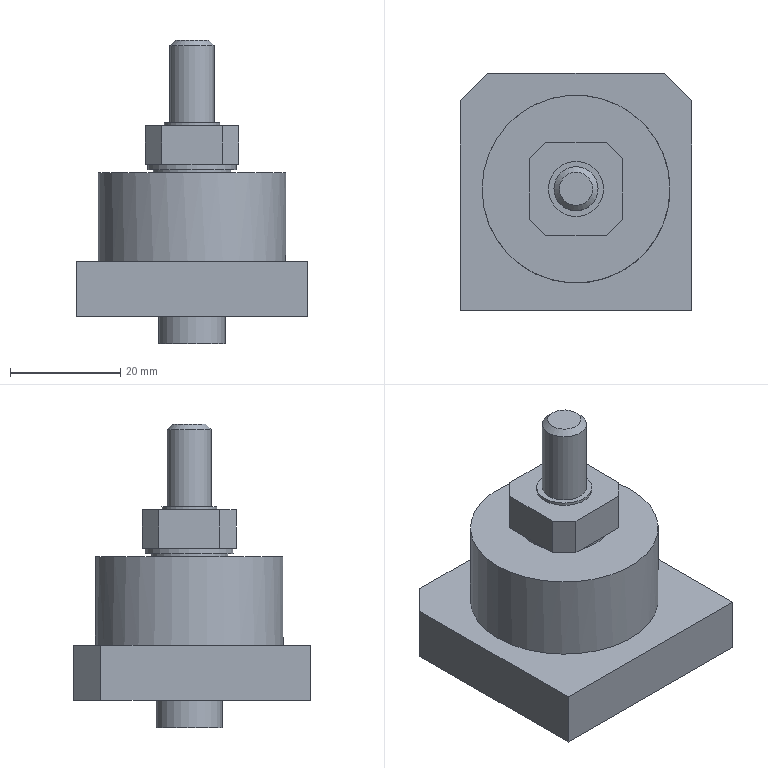Part | NX | features EXTRUDE 8, DATUM_CSYS 7, SKETCH 6, CHAMFER 3, OFFSET 1 | 1 solid | 30 faces | box 42 x 43 x 55 mm | volume 35859 mm3 | plane 23 | cylinder 6 | cone 1 | commonest cylinder face diameters 8 x1 10 x1 12 x1 14 x1 16 x1 34 x1
STEP:
#1=CARTESIAN_POINT('',(0.,16.,0.));
#2=VERTEX_POINT('',#1);
#3=CARTESIAN_POINT('',(0.,-22.,0.));
#4=VERTEX_POINT('',#3);
#5=CARTESIAN_POINT('',(0.,21.,0.));
#6=DIRECTION('',(0.,-1.,0.));
#7=VECTOR('',#6,1000.);
#8=LINE('',#5,#7);
#9=EDGE_CURVE('',#2,#4,#8,.T.);
#10=ORIENTED_EDGE('',*,*,#9,.F.);
#11=CARTESIAN_POINT('',(0.,16.,10.));
#12=VERTEX_POINT('',#11);
#13=CARTESIAN_POINT('',(0.,16.,10.));
#14=DIRECTION('',(0.,0.,1.));
#15=VECTOR('',#14,1000.);
#16=LINE('',#13,#15);
#17=EDGE_CURVE('',#2,#12,#16,.T.);
#18=ORIENTED_EDGE('',*,*,#17,.T.);
#19=CARTESIAN_POINT('',(0.,-22.,10.));
#20=VERTEX_POINT('',#19);
#21=CARTESIAN_POINT('',(0.,21.,10.));
#22=DIRECTION('',(0.,-1.,0.));
#23=VECTOR('',#22,1000.);
#24=LINE('',#21,#23);
#25=EDGE_CURVE('',#12,#20,#24,.T.);
#26=ORIENTED_EDGE('',*,*,#25,.T.);
#27=CARTESIAN_POINT('',(0.,-22.,10.));
#28=DIRECTION('',(0.,0.,-1.));
#29=VECTOR('',#28,1000.);
#30=LINE('',#27,#29);
#31=EDGE_CURVE('',#20,#4,#30,.T.);
#32=ORIENTED_EDGE('',*,*,#31,.T.);
#33=EDGE_LOOP('',(#10,#18,#26,#32));
#34=FACE_BOUND('',#33,.T.);
#35=CARTESIAN_POINT('',(0.,21.,10.));
#36=DIRECTION('',(1.,0.,0.));
#37=DIRECTION('',(0.,1.,0.));
#38=AXIS2_PLACEMENT_3D('',#35,#36,#37);
#39=PLANE('',#38);
#40=ADVANCED_FACE('',(#34),#39,.T.);
#41=CARTESIAN_POINT('',(-42.,-22.,0.));
#42=VERTEX_POINT('',#41);
#43=CARTESIAN_POINT('',(0.,-22.,0.));
#44=DIRECTION('',(-1.,0.,0.));
#45=VECTOR('',#44,1000.);
#46=LINE('',#43,#45);
#47=EDGE_CURVE('',#4,#42,#46,.T.);
#48=ORIENTED_EDGE('',*,*,#47,.F.);
#49=ORIENTED_EDGE('',*,*,#31,.F.);
#50=CARTESIAN_POINT('',(-42.,-22.,10.));
#51=VERTEX_POINT('',#50);
#52=CARTESIAN_POINT('',(0.,-22.,10.));
#53=DIRECTION('',(-1.,0.,0.));
#54=VECTOR('',#53,1000.);
#55=LINE('',#52,#54);
#56=EDGE_CURVE('',#20,#51,#55,.T.);
#57=ORIENTED_EDGE('',*,*,#56,.T.);
#58=CARTESIAN_POINT('',(-42.,-22.,10.));
#59=DIRECTION('',(0.,0.,-1.));
#60=VECTOR('',#59,1000.);
#61=LINE('',#58,#60);
#62=EDGE_CURVE('',#51,#42,#61,.T.);
#63=ORIENTED_EDGE('',*,*,#62,.T.);
#64=EDGE_LOOP('',(#48,#49,#57,#63));
#65=FACE_BOUND('',#64,.T.);
#66=CARTESIAN_POINT('',(0.,-22.,10.));
#67=DIRECTION('',(0.,-1.,0.));
#68=DIRECTION('',(1.,0.,0.));
#69=AXIS2_PLACEMENT_3D('',#66,#67,#68);
#70=PLANE('',#69);
#71=ADVANCED_FACE('',(#65),#70,.T.);
#72=CARTESIAN_POINT('',(-42.,16.,10.));
#73=VERTEX_POINT('',#72);
#74=CARTESIAN_POINT('',(-42.,-21.,10.));
#75=DIRECTION('',(0.,1.,0.));
#76=VECTOR('',#75,1000.);
#77=LINE('',#74,#76);
#78=EDGE_CURVE('',#51,#73,#77,.T.);
#79=ORIENTED_EDGE('',*,*,#78,.T.);
#80=CARTESIAN_POINT('',(-42.,16.,0.));
#81=VERTEX_POINT('',#80);
#82=CARTESIAN_POINT('',(-42.,16.,10.));
#83=DIRECTION('',(0.,0.,-1.));
#84=VECTOR('',#83,1000.);
#85=LINE('',#82,#84);
#86=EDGE_CURVE('',#73,#81,#85,.T.);
#87=ORIENTED_EDGE('',*,*,#86,.T.);
#88=CARTESIAN_POINT('',(-42.,-21.,0.));
#89=DIRECTION('',(0.,1.,0.));
#90=VECTOR('',#89,1000.);
#91=LINE('',#88,#90);
#92=EDGE_CURVE('',#42,#81,#91,.T.);
#93=ORIENTED_EDGE('',*,*,#92,.F.);
#94=ORIENTED_EDGE('',*,*,#62,.F.);
#95=EDGE_LOOP('',(#79,#87,#93,#94));
#96=FACE_BOUND('',#95,.T.);
#97=CARTESIAN_POINT('',(-42.,-21.,10.));
#98=DIRECTION('',(-1.,0.,0.));
#99=DIRECTION('',(0.,0.,1.));
#100=AXIS2_PLACEMENT_3D('',#97,#98,#99);
#101=PLANE('',#100);
#102=ADVANCED_FACE('',(#96),#101,.T.);
#103=CARTESIAN_POINT('',(-37.,21.,10.));
#104=VERTEX_POINT('',#103);
#105=CARTESIAN_POINT('',(-5.,21.,10.));
#106=VERTEX_POINT('',#105);
#107=CARTESIAN_POINT('',(-42.,21.,10.));
#108=DIRECTION('',(1.,0.,0.));
#109=VECTOR('',#108,1000.);
#110=LINE('',#107,#109);
#111=EDGE_CURVE('',#104,#106,#110,.T.);
#112=ORIENTED_EDGE('',*,*,#111,.T.);
#113=CARTESIAN_POINT('',(-5.,21.,0.));
#114=VERTEX_POINT('',#113);
#115=CARTESIAN_POINT('',(-5.,21.,10.));
#116=DIRECTION('',(0.,0.,-1.));
#117=VECTOR('',#116,1000.);
#118=LINE('',#115,#117);
#119=EDGE_CURVE('',#106,#114,#118,.T.);
#120=ORIENTED_EDGE('',*,*,#119,.T.);
#121=CARTESIAN_POINT('',(-37.,21.,0.));
#122=VERTEX_POINT('',#121);
#123=CARTESIAN_POINT('',(-42.,21.,0.));
#124=DIRECTION('',(1.,0.,0.));
#125=VECTOR('',#124,1000.);
#126=LINE('',#123,#125);
#127=EDGE_CURVE('',#122,#114,#126,.T.);
#128=ORIENTED_EDGE('',*,*,#127,.F.);
#129=CARTESIAN_POINT('',(-37.,21.,10.));
#130=DIRECTION('',(0.,0.,1.));
#131=VECTOR('',#130,1000.);
#132=LINE('',#129,#131);
#133=EDGE_CURVE('',#122,#104,#132,.T.);
#134=ORIENTED_EDGE('',*,*,#133,.T.);
#135=EDGE_LOOP('',(#112,#120,#128,#134));
#136=FACE_BOUND('',#135,.T.);
#137=CARTESIAN_POINT('',(-42.,21.,10.));
#138=DIRECTION('',(0.,1.,0.));
#139=DIRECTION('',(0.,0.,1.));
#140=AXIS2_PLACEMENT_3D('',#137,#138,#139);
#141=PLANE('',#140);
#142=ADVANCED_FACE('',(#136),#141,.T.);
#143=CARTESIAN_POINT('',(-38.,0.,10.));
#144=VERTEX_POINT('',#143);
#145=CARTESIAN_POINT('',(-21.,0.,10.));
#146=DIRECTION('',(0.,0.,-1.));
#147=DIRECTION('',(-1.,0.,0.));
#148=AXIS2_PLACEMENT_3D('',#145,#146,#147);
#149=CIRCLE('',#148,17.);
#150=EDGE_CURVE('',#144,#144,#149,.T.);
#151=ORIENTED_EDGE('',*,*,#150,.T.);
#152=EDGE_LOOP('',(#151));
#153=FACE_BOUND('',#152,.T.);
#154=ORIENTED_EDGE('',*,*,#25,.F.);
#155=CARTESIAN_POINT('',(-5.,21.,10.));
#156=DIRECTION('',(0.7071,-0.7071,0.));
#157=VECTOR('',#156,1000.);
#158=LINE('',#155,#157);
#159=EDGE_CURVE('',#12,#106,#158,.F.);
#160=ORIENTED_EDGE('',*,*,#159,.T.);
#161=ORIENTED_EDGE('',*,*,#111,.F.);
#162=CARTESIAN_POINT('',(-42.,16.,10.));
#163=DIRECTION('',(0.7071,0.7071,0.));
#164=VECTOR('',#163,1000.);
#165=LINE('',#162,#164);
#166=EDGE_CURVE('',#104,#73,#165,.F.);
#167=ORIENTED_EDGE('',*,*,#166,.T.);
#168=ORIENTED_EDGE('',*,*,#78,.F.);
#169=ORIENTED_EDGE('',*,*,#56,.F.);
#170=EDGE_LOOP('',(#154,#160,#161,#167,#168,#169));
#171=FACE_BOUND('',#170,.T.);
#172=CARTESIAN_POINT('',(0.,0.,10.));
#173=DIRECTION('',(0.,0.,-1.));
#174=DIRECTION('',(-1.,0.,0.));
#175=AXIS2_PLACEMENT_3D('',#172,#173,#174);
#176=PLANE('',#175);
#177=ADVANCED_FACE('',(#153,#171),#176,.F.);
#178=CARTESIAN_POINT('',(-27.,0.,0.));
#179=VERTEX_POINT('',#178);
#180=CARTESIAN_POINT('',(-21.,0.,0.));
#181=DIRECTION('',(0.,0.,-1.));
#182=DIRECTION('',(-1.,0.,0.));
#183=AXIS2_PLACEMENT_3D('',#180,#181,#182);
#184=CIRCLE('',#183,6.);
#185=EDGE_CURVE('',#179,#179,#184,.F.);
#186=ORIENTED_EDGE('',*,*,#185,.T.);
#187=EDGE_LOOP('',(#186));
#188=FACE_BOUND('',#187,.T.);
#189=ORIENTED_EDGE('',*,*,#127,.T.);
#190=CARTESIAN_POINT('',(8.,8.,0.));
#191=DIRECTION('',(-0.7071,0.7071,0.));
#192=VECTOR('',#191,1000.);
#193=LINE('',#190,#192);
#194=EDGE_CURVE('',#114,#2,#193,.F.);
#195=ORIENTED_EDGE('',*,*,#194,.T.);
#196=ORIENTED_EDGE('',*,*,#9,.T.);
#197=ORIENTED_EDGE('',*,*,#47,.T.);
#198=ORIENTED_EDGE('',*,*,#92,.T.);
#199=CARTESIAN_POINT('',(-29.,29.,0.));
#200=DIRECTION('',(-0.7071,-0.7071,0.));
#201=VECTOR('',#200,1000.);
#202=LINE('',#199,#201);
#203=EDGE_CURVE('',#81,#122,#202,.F.);
#204=ORIENTED_EDGE('',*,*,#203,.T.);
#205=EDGE_LOOP('',(#189,#195,#196,#197,#198,#204));
#206=FACE_BOUND('',#205,.T.);
#207=CARTESIAN_POINT('',(0.,0.,0.));
#208=DIRECTION('',(0.,0.,-1.));
#209=DIRECTION('',(-1.,0.,0.));
#210=AXIS2_PLACEMENT_3D('',#207,#208,#209);
#211=PLANE('',#210);
#212=ADVANCED_FACE('',(#188,#206),#211,.T.);
#213=CARTESIAN_POINT('',(-4.,0.,26.));
#214=VERTEX_POINT('',#213);
#215=CARTESIAN_POINT('',(-21.,0.,26.));
#216=DIRECTION('',(0.,0.,-1.));
#217=DIRECTION('',(1.,0.,0.));
#218=AXIS2_PLACEMENT_3D('',#215,#216,#217);
#219=CIRCLE('',#218,17.);
#220=EDGE_CURVE('',#214,#214,#219,.T.);
#221=ORIENTED_EDGE('',*,*,#220,.T.);
#222=EDGE_LOOP('',(#221));
#223=FACE_BOUND('',#222,.T.);
#224=ORIENTED_EDGE('',*,*,#150,.F.);
#225=EDGE_LOOP('',(#224));
#226=FACE_BOUND('',#225,.T.);
#227=CARTESIAN_POINT('',(-21.,0.,26.));
#228=DIRECTION('',(0.,0.,-1.));
#229=DIRECTION('',(-1.,0.,0.));
#230=AXIS2_PLACEMENT_3D('',#227,#228,#229);
#231=CYLINDRICAL_SURFACE('',#230,17.);
#232=ADVANCED_FACE('',(#223,#226),#231,.T.);
#233=CARTESIAN_POINT('',(-14.,0.,26.));
#234=VERTEX_POINT('',#233);
#235=CARTESIAN_POINT('',(-21.,0.,26.));
#236=DIRECTION('',(0.,0.,1.));
#237=DIRECTION('',(1.,0.,0.));
#238=AXIS2_PLACEMENT_3D('',#235,#236,#237);
#239=CIRCLE('',#238,7.);
#240=EDGE_CURVE('',#234,#234,#239,.T.);
#241=ORIENTED_EDGE('',*,*,#240,.F.);
#242=EDGE_LOOP('',(#241));
#243=FACE_BOUND('',#242,.T.);
#244=ORIENTED_EDGE('',*,*,#220,.F.);
#245=EDGE_LOOP('',(#244));
#246=FACE_BOUND('',#245,.T.);
#247=CARTESIAN_POINT('',(-21.,0.,26.));
#248=DIRECTION('',(0.,0.,-1.));
#249=DIRECTION('',(-1.,0.,0.));
#250=AXIS2_PLACEMENT_3D('',#247,#248,#249);
#251=PLANE('',#250);
#252=ADVANCED_FACE('',(#243,#246),#251,.F.);
#253=CARTESIAN_POINT('',(-27.,0.,-5.));
#254=VERTEX_POINT('',#253);
#255=CARTESIAN_POINT('',(-21.,0.,-5.));
#256=DIRECTION('',(0.,0.,-1.));
#257=DIRECTION('',(-1.,0.,0.));
#258=AXIS2_PLACEMENT_3D('',#255,#256,#257);
#259=CIRCLE('',#258,6.);
#260=EDGE_CURVE('',#254,#254,#259,.F.);
#261=ORIENTED_EDGE('',*,*,#260,.T.);
#262=EDGE_LOOP('',(#261));
#263=FACE_BOUND('',#262,.T.);
#264=ORIENTED_EDGE('',*,*,#185,.F.);
#265=EDGE_LOOP('',(#264));
#266=FACE_BOUND('',#265,.T.);
#267=CARTESIAN_POINT('',(-21.,0.,-5.));
#268=DIRECTION('',(0.,0.,1.));
#269=DIRECTION('',(1.,0.,0.));
#270=AXIS2_PLACEMENT_3D('',#267,#268,#269);
#271=CYLINDRICAL_SURFACE('',#270,6.);
#272=ADVANCED_FACE('',(#263,#266),#271,.T.);
#273=ORIENTED_EDGE('',*,*,#260,.F.);
#274=EDGE_LOOP('',(#273));
#275=FACE_BOUND('',#274,.T.);
#276=CARTESIAN_POINT('',(-21.,0.,-5.));
#277=DIRECTION('',(0.,0.,-1.));
#278=DIRECTION('',(-1.,0.,0.));
#279=AXIS2_PLACEMENT_3D('',#276,#277,#278);
#280=PLANE('',#279);
#281=ADVANCED_FACE('',(#275),#280,.T.);
#282=CARTESIAN_POINT('',(-14.,0.,26.5));
#283=VERTEX_POINT('',#282);
#284=CARTESIAN_POINT('',(-21.,0.,26.5));
#285=DIRECTION('',(0.,0.,1.));
#286=DIRECTION('',(1.,0.,0.));
#287=AXIS2_PLACEMENT_3D('',#284,#285,#286);
#288=CIRCLE('',#287,7.);
#289=EDGE_CURVE('',#283,#283,#288,.T.);
#290=ORIENTED_EDGE('',*,*,#289,.F.);
#291=EDGE_LOOP('',(#290));
#292=FACE_BOUND('',#291,.T.);
#293=ORIENTED_EDGE('',*,*,#240,.T.);
#294=EDGE_LOOP('',(#293));
#295=FACE_BOUND('',#294,.T.);
#296=CARTESIAN_POINT('',(-21.,0.,26.5));
#297=DIRECTION('',(0.,0.,-1.));
#298=DIRECTION('',(-1.,0.,0.));
#299=AXIS2_PLACEMENT_3D('',#296,#297,#298);
#300=CYLINDRICAL_SURFACE('',#299,7.);
#301=ADVANCED_FACE('',(#292,#295),#300,.T.);
#302=CARTESIAN_POINT('',(-13.,0.,27.5));
#303=VERTEX_POINT('',#302);
#304=CARTESIAN_POINT('',(-21.,0.,27.5));
#305=DIRECTION('',(0.,0.,-1.));
#306=DIRECTION('',(1.,0.,0.));
#307=AXIS2_PLACEMENT_3D('',#304,#305,#306);
#308=CIRCLE('',#307,8.);
#309=EDGE_CURVE('',#303,#303,#308,.T.);
#310=ORIENTED_EDGE('',*,*,#309,.T.);
#311=EDGE_LOOP('',(#310));
#312=FACE_BOUND('',#311,.T.);
#313=CARTESIAN_POINT('',(-13.,0.,26.5));
#314=VERTEX_POINT('',#313);
#315=CARTESIAN_POINT('',(-21.,0.,26.5));
#316=DIRECTION('',(0.,0.,-1.));
#317=DIRECTION('',(1.,0.,0.));
#318=AXIS2_PLACEMENT_3D('',#315,#316,#317);
#319=CIRCLE('',#318,8.);
#320=EDGE_CURVE('',#314,#314,#319,.T.);
#321=ORIENTED_EDGE('',*,*,#320,.F.);
#322=EDGE_LOOP('',(#321));
#323=FACE_BOUND('',#322,.T.);
#324=CARTESIAN_POINT('',(-21.,0.,27.5));
#325=DIRECTION('',(0.,0.,-1.));
#326=DIRECTION('',(-1.,0.,0.));
#327=AXIS2_PLACEMENT_3D('',#324,#325,#326);
#328=CYLINDRICAL_SURFACE('',#327,8.);
#329=ADVANCED_FACE('',(#312,#323),#328,.T.);
#330=ORIENTED_EDGE('',*,*,#289,.T.);
#331=EDGE_LOOP('',(#330));
#332=FACE_BOUND('',#331,.T.);
#333=ORIENTED_EDGE('',*,*,#320,.T.);
#334=EDGE_LOOP('',(#333));
#335=FACE_BOUND('',#334,.T.);
#336=CARTESIAN_POINT('',(-21.,0.,26.5));
#337=DIRECTION('',(0.,0.,-1.));
#338=DIRECTION('',(-1.,0.,0.));
#339=AXIS2_PLACEMENT_3D('',#336,#337,#338);
#340=PLANE('',#339);
#341=ADVANCED_FACE('',(#332,#335),#340,.T.);
#342=CARTESIAN_POINT('',(-29.5,5.5,27.5));
#343=VERTEX_POINT('',#342);
#344=CARTESIAN_POINT('',(-29.5,-5.5,27.5));
#345=VERTEX_POINT('',#344);
#346=CARTESIAN_POINT('',(-29.5,8.5,27.5));
#347=DIRECTION('',(0.,-1.,0.));
#348=VECTOR('',#347,1000.);
#349=LINE('',#346,#348);
#350=EDGE_CURVE('',#343,#345,#349,.T.);
#351=ORIENTED_EDGE('',*,*,#350,.T.);
#352=CARTESIAN_POINT('',(-29.5,-5.5,34.5));
#353=VERTEX_POINT('',#352);
#354=CARTESIAN_POINT('',(-29.5,-5.5,34.5));
#355=DIRECTION('',(0.,0.,1.));
#356=VECTOR('',#355,1000.);
#357=LINE('',#354,#356);
#358=EDGE_CURVE('',#345,#353,#357,.T.);
#359=ORIENTED_EDGE('',*,*,#358,.T.);
#360=CARTESIAN_POINT('',(-29.5,5.5,34.5));
#361=VERTEX_POINT('',#360);
#362=CARTESIAN_POINT('',(-29.5,8.5,34.5));
#363=DIRECTION('',(0.,-1.,0.));
#364=VECTOR('',#363,1000.);
#365=LINE('',#362,#364);
#366=EDGE_CURVE('',#361,#353,#365,.T.);
#367=ORIENTED_EDGE('',*,*,#366,.F.);
#368=CARTESIAN_POINT('',(-29.5,5.5,34.5));
#369=DIRECTION('',(0.,0.,-1.));
#370=VECTOR('',#369,1000.);
#371=LINE('',#368,#370);
#372=EDGE_CURVE('',#361,#343,#371,.T.);
#373=ORIENTED_EDGE('',*,*,#372,.T.);
#374=EDGE_LOOP('',(#351,#359,#367,#373));
#375=FACE_BOUND('',#374,.T.);
#376=CARTESIAN_POINT('',(-29.5,8.5,34.5));
#377=DIRECTION('',(1.,0.,0.));
#378=DIRECTION('',(0.,1.,0.));
#379=AXIS2_PLACEMENT_3D('',#376,#377,#378);
#380=PLANE('',#379);
#381=ADVANCED_FACE('',(#375),#380,.F.);
#382=CARTESIAN_POINT('',(-26.5,-8.5,27.5));
#383=VERTEX_POINT('',#382);
#384=CARTESIAN_POINT('',(-15.5,-8.5,27.5));
#385=VERTEX_POINT('',#384);
#386=CARTESIAN_POINT('',(-29.5,-8.5,27.5));
#387=DIRECTION('',(1.,0.,0.));
#388=VECTOR('',#387,1000.);
#389=LINE('',#386,#388);
#390=EDGE_CURVE('',#383,#385,#389,.T.);
#391=ORIENTED_EDGE('',*,*,#390,.T.);
#392=CARTESIAN_POINT('',(-15.5,-8.5,34.5));
#393=VERTEX_POINT('',#392);
#394=CARTESIAN_POINT('',(-15.5,-8.5,34.5));
#395=DIRECTION('',(0.,0.,1.));
#396=VECTOR('',#395,1000.);
#397=LINE('',#394,#396);
#398=EDGE_CURVE('',#385,#393,#397,.T.);
#399=ORIENTED_EDGE('',*,*,#398,.T.);
#400=CARTESIAN_POINT('',(-26.5,-8.5,34.5));
#401=VERTEX_POINT('',#400);
#402=CARTESIAN_POINT('',(-29.5,-8.5,34.5));
#403=DIRECTION('',(1.,0.,0.));
#404=VECTOR('',#403,1000.);
#405=LINE('',#402,#404);
#406=EDGE_CURVE('',#401,#393,#405,.T.);
#407=ORIENTED_EDGE('',*,*,#406,.F.);
#408=CARTESIAN_POINT('',(-26.5,-8.5,34.5));
#409=DIRECTION('',(0.,0.,-1.));
#410=VECTOR('',#409,1000.);
#411=LINE('',#408,#410);
#412=EDGE_CURVE('',#401,#383,#411,.T.);
#413=ORIENTED_EDGE('',*,*,#412,.T.);
#414=EDGE_LOOP('',(#391,#399,#407,#413));
#415=FACE_BOUND('',#414,.T.);
#416=CARTESIAN_POINT('',(-29.5,-8.5,34.5));
#417=DIRECTION('',(0.,1.,0.));
#418=DIRECTION('',(0.,0.,1.));
#419=AXIS2_PLACEMENT_3D('',#416,#417,#418);
#420=PLANE('',#419);
#421=ADVANCED_FACE('',(#415),#420,.F.);
#422=CARTESIAN_POINT('',(-12.5,-5.5,27.5));
#423=VERTEX_POINT('',#422);
#424=CARTESIAN_POINT('',(-12.5,5.5,27.5));
#425=VERTEX_POINT('',#424);
#426=CARTESIAN_POINT('',(-12.5,-8.5,27.5));
#427=DIRECTION('',(0.,1.,0.));
#428=VECTOR('',#427,1000.);
#429=LINE('',#426,#428);
#430=EDGE_CURVE('',#423,#425,#429,.T.);
#431=ORIENTED_EDGE('',*,*,#430,.T.);
#432=CARTESIAN_POINT('',(-12.5,5.5,34.5));
#433=VERTEX_POINT('',#432);
#434=CARTESIAN_POINT('',(-12.5,5.5,34.5));
#435=DIRECTION('',(0.,0.,1.));
#436=VECTOR('',#435,1000.);
#437=LINE('',#434,#436);
#438=EDGE_CURVE('',#425,#433,#437,.T.);
#439=ORIENTED_EDGE('',*,*,#438,.T.);
#440=CARTESIAN_POINT('',(-12.5,-5.5,34.5));
#441=VERTEX_POINT('',#440);
#442=CARTESIAN_POINT('',(-12.5,-8.5,34.5));
#443=DIRECTION('',(0.,1.,0.));
#444=VECTOR('',#443,1000.);
#445=LINE('',#442,#444);
#446=EDGE_CURVE('',#441,#433,#445,.T.);
#447=ORIENTED_EDGE('',*,*,#446,.F.);
#448=CARTESIAN_POINT('',(-12.5,-5.5,34.5));
#449=DIRECTION('',(0.,0.,-1.));
#450=VECTOR('',#449,1000.);
#451=LINE('',#448,#450);
#452=EDGE_CURVE('',#441,#423,#451,.T.);
#453=ORIENTED_EDGE('',*,*,#452,.T.);
#454=EDGE_LOOP('',(#431,#439,#447,#453));
#455=FACE_BOUND('',#454,.T.);
#456=CARTESIAN_POINT('',(-12.5,-8.5,34.5));
#457=DIRECTION('',(-1.,0.,0.));
#458=DIRECTION('',(0.,-1.,0.));
#459=AXIS2_PLACEMENT_3D('',#456,#457,#458);
#460=PLANE('',#459);
#461=ADVANCED_FACE('',(#455),#460,.F.);
#462=CARTESIAN_POINT('',(-15.5,8.5,34.5));
#463=VERTEX_POINT('',#462);
#464=CARTESIAN_POINT('',(-26.5,8.5,34.5));
#465=VERTEX_POINT('',#464);
#466=CARTESIAN_POINT('',(-12.5,8.5,34.5));
#467=DIRECTION('',(-1.,0.,0.));
#468=VECTOR('',#467,1000.);
#469=LINE('',#466,#468);
#470=EDGE_CURVE('',#463,#465,#469,.T.);
#471=ORIENTED_EDGE('',*,*,#470,.F.);
#472=CARTESIAN_POINT('',(-15.5,8.5,27.5));
#473=VERTEX_POINT('',#472);
#474=CARTESIAN_POINT('',(-15.5,8.5,34.5));
#475=DIRECTION('',(0.,0.,-1.));
#476=VECTOR('',#475,1000.);
#477=LINE('',#474,#476);
#478=EDGE_CURVE('',#463,#473,#477,.T.);
#479=ORIENTED_EDGE('',*,*,#478,.T.);
#480=CARTESIAN_POINT('',(-26.5,8.5,27.5));
#481=VERTEX_POINT('',#480);
#482=CARTESIAN_POINT('',(-12.5,8.5,27.5));
#483=DIRECTION('',(-1.,0.,0.));
#484=VECTOR('',#483,1000.);
#485=LINE('',#482,#484);
#486=EDGE_CURVE('',#473,#481,#485,.T.);
#487=ORIENTED_EDGE('',*,*,#486,.T.);
#488=CARTESIAN_POINT('',(-26.5,8.5,34.5));
#489=DIRECTION('',(0.,0.,1.));
#490=VECTOR('',#489,1000.);
#491=LINE('',#488,#490);
#492=EDGE_CURVE('',#481,#465,#491,.T.);
#493=ORIENTED_EDGE('',*,*,#492,.T.);
#494=EDGE_LOOP('',(#471,#479,#487,#493));
#495=FACE_BOUND('',#494,.T.);
#496=CARTESIAN_POINT('',(-12.5,8.5,34.5));
#497=DIRECTION('',(0.,-1.,0.));
#498=DIRECTION('',(0.,0.,-1.));
#499=AXIS2_PLACEMENT_3D('',#496,#497,#498);
#500=PLANE('',#499);
#501=ADVANCED_FACE('',(#495),#500,.F.);
#502=CARTESIAN_POINT('',(-16.,0.,34.5));
#503=VERTEX_POINT('',#502);
#504=CARTESIAN_POINT('',(-21.,0.,34.5));
#505=DIRECTION('',(0.,0.,1.));
#506=DIRECTION('',(1.,0.,0.));
#507=AXIS2_PLACEMENT_3D('',#504,#505,#506);
#508=CIRCLE('',#507,5.);
#509=EDGE_CURVE('',#503,#503,#508,.T.);
#510=ORIENTED_EDGE('',*,*,#509,.F.);
#511=EDGE_LOOP('',(#510));
#512=FACE_BOUND('',#511,.T.);
#513=ORIENTED_EDGE('',*,*,#446,.T.);
#514=CARTESIAN_POINT('',(-3.5,-3.5,34.5));
#515=DIRECTION('',(0.7071,-0.7071,0.));
#516=VECTOR('',#515,1000.);
#517=LINE('',#514,#516);
#518=EDGE_CURVE('',#433,#463,#517,.F.);
#519=ORIENTED_EDGE('',*,*,#518,.T.);
#520=ORIENTED_EDGE('',*,*,#470,.T.);
#521=CARTESIAN_POINT('',(-17.5,17.5,34.5));
#522=DIRECTION('',(0.7071,0.7071,0.));
#523=VECTOR('',#522,1000.);
#524=LINE('',#521,#523);
#525=EDGE_CURVE('',#465,#361,#524,.F.);
#526=ORIENTED_EDGE('',*,*,#525,.T.);
#527=ORIENTED_EDGE('',*,*,#366,.T.);
#528=CARTESIAN_POINT('',(-17.5,-17.5,34.5));
#529=DIRECTION('',(-0.7071,0.7071,0.));
#530=VECTOR('',#529,1000.);
#531=LINE('',#528,#530);
#532=EDGE_CURVE('',#353,#401,#531,.F.);
#533=ORIENTED_EDGE('',*,*,#532,.T.);
#534=ORIENTED_EDGE('',*,*,#406,.T.);
#535=CARTESIAN_POINT('',(-3.5,3.5,34.5));
#536=DIRECTION('',(-0.7071,-0.7071,0.));
#537=VECTOR('',#536,1000.);
#538=LINE('',#535,#537);
#539=EDGE_CURVE('',#393,#441,#538,.F.);
#540=ORIENTED_EDGE('',*,*,#539,.T.);
#541=EDGE_LOOP('',(#513,#519,#520,#526,#527,#533,#534,#540));
#542=FACE_BOUND('',#541,.T.);
#543=CARTESIAN_POINT('',(0.,0.,34.5));
#544=DIRECTION('',(0.,0.,1.));
#545=DIRECTION('',(1.,0.,0.));
#546=AXIS2_PLACEMENT_3D('',#543,#544,#545);
#547=PLANE('',#546);
#548=ADVANCED_FACE('',(#512,#542),#547,.T.);
#549=ORIENTED_EDGE('',*,*,#309,.F.);
#550=EDGE_LOOP('',(#549));
#551=FACE_BOUND('',#550,.T.);
#552=ORIENTED_EDGE('',*,*,#486,.F.);
#553=CARTESIAN_POINT('',(-15.5,8.5,27.5));
#554=DIRECTION('',(-0.7071,0.7071,0.));
#555=VECTOR('',#554,1000.);
#556=LINE('',#553,#555);
#557=EDGE_CURVE('',#473,#425,#556,.F.);
#558=ORIENTED_EDGE('',*,*,#557,.T.);
#559=ORIENTED_EDGE('',*,*,#430,.F.);
#560=CARTESIAN_POINT('',(-12.5,-5.5,27.5));
#561=DIRECTION('',(0.7071,0.7071,0.));
#562=VECTOR('',#561,1000.);
#563=LINE('',#560,#562);
#564=EDGE_CURVE('',#423,#385,#563,.F.);
#565=ORIENTED_EDGE('',*,*,#564,.T.);
#566=ORIENTED_EDGE('',*,*,#390,.F.);
#567=CARTESIAN_POINT('',(-26.5,-8.5,27.5));
#568=DIRECTION('',(0.7071,-0.7071,0.));
#569=VECTOR('',#568,1000.);
#570=LINE('',#567,#569);
#571=EDGE_CURVE('',#383,#345,#570,.F.);
#572=ORIENTED_EDGE('',*,*,#571,.T.);
#573=ORIENTED_EDGE('',*,*,#350,.F.);
#574=CARTESIAN_POINT('',(-29.5,5.5,27.5));
#575=DIRECTION('',(-0.7071,-0.7071,0.));
#576=VECTOR('',#575,1000.);
#577=LINE('',#574,#576);
#578=EDGE_CURVE('',#343,#481,#577,.F.);
#579=ORIENTED_EDGE('',*,*,#578,.T.);
#580=EDGE_LOOP('',(#552,#558,#559,#565,#566,#572,#573,#579));
#581=FACE_BOUND('',#580,.T.);
#582=CARTESIAN_POINT('',(0.,0.,27.5));
#583=DIRECTION('',(0.,0.,1.));
#584=DIRECTION('',(1.,0.,0.));
#585=AXIS2_PLACEMENT_3D('',#582,#583,#584);
#586=PLANE('',#585);
#587=ADVANCED_FACE('',(#551,#581),#586,.F.);
#588=ORIENTED_EDGE('',*,*,#518,.F.);
#589=ORIENTED_EDGE('',*,*,#438,.F.);
#590=ORIENTED_EDGE('',*,*,#557,.F.);
#591=ORIENTED_EDGE('',*,*,#478,.F.);
#592=EDGE_LOOP('',(#588,#589,#590,#591));
#593=FACE_BOUND('',#592,.T.);
#594=CARTESIAN_POINT('',(-15.5,8.5,34.5));
#595=DIRECTION('',(-0.7071,-0.7071,0.));
#596=DIRECTION('',(0.,0.,-1.));
#597=AXIS2_PLACEMENT_3D('',#594,#595,#596);
#598=PLANE('',#597);
#599=ADVANCED_FACE('',(#593),#598,.F.);
#600=ORIENTED_EDGE('',*,*,#539,.F.);
#601=ORIENTED_EDGE('',*,*,#398,.F.);
#602=ORIENTED_EDGE('',*,*,#564,.F.);
#603=ORIENTED_EDGE('',*,*,#452,.F.);
#604=EDGE_LOOP('',(#600,#601,#602,#603));
#605=FACE_BOUND('',#604,.T.);
#606=CARTESIAN_POINT('',(-12.5,-5.5,34.5));
#607=DIRECTION('',(-0.7071,0.7071,0.));
#608=DIRECTION('',(0.,0.,-1.));
#609=AXIS2_PLACEMENT_3D('',#606,#607,#608);
#610=PLANE('',#609);
#611=ADVANCED_FACE('',(#605),#610,.F.);
#612=ORIENTED_EDGE('',*,*,#532,.F.);
#613=ORIENTED_EDGE('',*,*,#358,.F.);
#614=ORIENTED_EDGE('',*,*,#571,.F.);
#615=ORIENTED_EDGE('',*,*,#412,.F.);
#616=EDGE_LOOP('',(#612,#613,#614,#615));
#617=FACE_BOUND('',#616,.T.);
#618=CARTESIAN_POINT('',(-26.5,-8.5,34.5));
#619=DIRECTION('',(0.7071,0.7071,0.));
#620=DIRECTION('',(0.,0.,-1.));
#621=AXIS2_PLACEMENT_3D('',#618,#619,#620);
#622=PLANE('',#621);
#623=ADVANCED_FACE('',(#617),#622,.F.);
#624=ORIENTED_EDGE('',*,*,#525,.F.);
#625=ORIENTED_EDGE('',*,*,#492,.F.);
#626=ORIENTED_EDGE('',*,*,#578,.F.);
#627=ORIENTED_EDGE('',*,*,#372,.F.);
#628=EDGE_LOOP('',(#624,#625,#626,#627));
#629=FACE_BOUND('',#628,.T.);
#630=CARTESIAN_POINT('',(-29.5,5.5,34.5));
#631=DIRECTION('',(0.7071,-0.7071,0.));
#632=DIRECTION('',(0.,0.,-1.));
#633=AXIS2_PLACEMENT_3D('',#630,#631,#632);
#634=PLANE('',#633);
#635=ADVANCED_FACE('',(#629),#634,.F.);
#636=ORIENTED_EDGE('',*,*,#159,.F.);
#637=ORIENTED_EDGE('',*,*,#17,.F.);
#638=ORIENTED_EDGE('',*,*,#194,.F.);
#639=ORIENTED_EDGE('',*,*,#119,.F.);
#640=EDGE_LOOP('',(#636,#637,#638,#639));
#641=FACE_BOUND('',#640,.T.);
#642=CARTESIAN_POINT('',(-5.,21.,10.));
#643=DIRECTION('',(-0.7071,-0.7071,0.));
#644=DIRECTION('',(0.,0.,-1.));
#645=AXIS2_PLACEMENT_3D('',#642,#643,#644);
#646=PLANE('',#645);
#647=ADVANCED_FACE('',(#641),#646,.F.);
#648=ORIENTED_EDGE('',*,*,#166,.F.);
#649=ORIENTED_EDGE('',*,*,#133,.F.);
#650=ORIENTED_EDGE('',*,*,#203,.F.);
#651=ORIENTED_EDGE('',*,*,#86,.F.);
#652=EDGE_LOOP('',(#648,#649,#650,#651));
#653=FACE_BOUND('',#652,.T.);
#654=CARTESIAN_POINT('',(-42.,16.,10.));
#655=DIRECTION('',(0.7071,-0.7071,0.));
#656=DIRECTION('',(0.,0.,-1.));
#657=AXIS2_PLACEMENT_3D('',#654,#655,#656);
#658=PLANE('',#657);
#659=ADVANCED_FACE('',(#653),#658,.F.);
#660=CARTESIAN_POINT('',(-16.,0.,35.));
#661=VERTEX_POINT('',#660);
#662=CARTESIAN_POINT('',(-21.,0.,35.));
#663=DIRECTION('',(0.,0.,1.));
#664=DIRECTION('',(1.,0.,0.));
#665=AXIS2_PLACEMENT_3D('',#662,#663,#664);
#666=CIRCLE('',#665,5.);
#667=EDGE_CURVE('',#661,#661,#666,.T.);
#668=ORIENTED_EDGE('',*,*,#667,.F.);
#669=EDGE_LOOP('',(#668));
#670=FACE_BOUND('',#669,.T.);
#671=ORIENTED_EDGE('',*,*,#509,.T.);
#672=EDGE_LOOP('',(#671));
#673=FACE_BOUND('',#672,.T.);
#674=CARTESIAN_POINT('',(-21.,0.,35.));
#675=DIRECTION('',(0.,0.,-1.));
#676=DIRECTION('',(-1.,0.,0.));
#677=AXIS2_PLACEMENT_3D('',#674,#675,#676);
#678=CYLINDRICAL_SURFACE('',#677,5.);
#679=ADVANCED_FACE('',(#670,#673),#678,.T.);
#680=CARTESIAN_POINT('',(-17.,0.,35.));
#681=VERTEX_POINT('',#680);
#682=CARTESIAN_POINT('',(-21.,0.,35.));
#683=DIRECTION('',(0.,0.,1.));
#684=DIRECTION('',(1.,0.,0.));
#685=AXIS2_PLACEMENT_3D('',#682,#683,#684);
#686=CIRCLE('',#685,4.);
#687=EDGE_CURVE('',#681,#681,#686,.T.);
#688=ORIENTED_EDGE('',*,*,#687,.F.);
#689=EDGE_LOOP('',(#688));
#690=FACE_BOUND('',#689,.T.);
#691=ORIENTED_EDGE('',*,*,#667,.T.);
#692=EDGE_LOOP('',(#691));
#693=FACE_BOUND('',#692,.T.);
#694=CARTESIAN_POINT('',(-21.,0.,35.));
#695=DIRECTION('',(0.,0.,1.));
#696=DIRECTION('',(1.,0.,0.));
#697=AXIS2_PLACEMENT_3D('',#694,#695,#696);
#698=PLANE('',#697);
#699=ADVANCED_FACE('',(#690,#693),#698,.T.);
#700=CARTESIAN_POINT('',(-17.,0.,49.));
#701=VERTEX_POINT('',#700);
#702=CARTESIAN_POINT('',(-21.,0.,49.));
#703=DIRECTION('',(0.,0.,1.));
#704=DIRECTION('',(1.,0.,0.));
#705=AXIS2_PLACEMENT_3D('',#702,#703,#704);
#706=CIRCLE('',#705,4.);
#707=EDGE_CURVE('',#701,#701,#706,.F.);
#708=ORIENTED_EDGE('',*,*,#707,.T.);
#709=EDGE_LOOP('',(#708));
#710=FACE_BOUND('',#709,.T.);
#711=ORIENTED_EDGE('',*,*,#687,.T.);
#712=EDGE_LOOP('',(#711));
#713=FACE_BOUND('',#712,.T.);
#714=CARTESIAN_POINT('',(-21.,0.,50.));
#715=DIRECTION('',(0.,0.,-1.));
#716=DIRECTION('',(-1.,0.,0.));
#717=AXIS2_PLACEMENT_3D('',#714,#715,#716);
#718=CYLINDRICAL_SURFACE('',#717,4.);
#719=ADVANCED_FACE('',(#710,#713),#718,.T.);
#720=CARTESIAN_POINT('',(-18.,0.,50.));
#721=VERTEX_POINT('',#720);
#722=CARTESIAN_POINT('',(-21.,0.,50.));
#723=DIRECTION('',(0.,0.,1.));
#724=DIRECTION('',(1.,0.,0.));
#725=AXIS2_PLACEMENT_3D('',#722,#723,#724);
#726=CIRCLE('',#725,3.);
#727=EDGE_CURVE('',#721,#721,#726,.T.);
#728=ORIENTED_EDGE('',*,*,#727,.T.);
#729=EDGE_LOOP('',(#728));
#730=FACE_BOUND('',#729,.T.);
#731=CARTESIAN_POINT('',(-21.,0.,50.));
#732=DIRECTION('',(0.,0.,1.));
#733=DIRECTION('',(1.,0.,0.));
#734=AXIS2_PLACEMENT_3D('',#731,#732,#733);
#735=PLANE('',#734);
#736=ADVANCED_FACE('',(#730),#735,.T.);
#737=ORIENTED_EDGE('',*,*,#707,.F.);
#738=EDGE_LOOP('',(#737));
#739=FACE_BOUND('',#738,.T.);
#740=ORIENTED_EDGE('',*,*,#727,.F.);
#741=EDGE_LOOP('',(#740));
#742=FACE_BOUND('',#741,.T.);
#743=CARTESIAN_POINT('',(-21.,0.,50.));
#744=DIRECTION('',(0.,0.,-1.));
#745=DIRECTION('',(-1.,0.,0.));
#746=AXIS2_PLACEMENT_3D('',#743,#744,#745);
#747=CONICAL_SURFACE('',#746,3.,0.7854);
#748=ADVANCED_FACE('',(#739,#742),#747,.T.);
#749=CLOSED_SHELL('',(#40,#71,#102,#142,#177,#212,#232,#252,#272,#281,#301,#329,#341,#381,#421,#461,#501,#548,#587,#599,#611,#623,#635,#647,#659,#679,#699,#719,#736,#748));
#750=MANIFOLD_SOLID_BREP('',#749);
#751=(LENGTH_UNIT()NAMED_UNIT(*)SI_UNIT(.MILLI.,.METRE.));
#752=UNCERTAINTY_MEASURE_WITH_UNIT(LENGTH_MEASURE(0.00001),#751,'','');
#753=(NAMED_UNIT(*)PLANE_ANGLE_UNIT()SI_UNIT($,.RADIAN.));
#754=(NAMED_UNIT(*)SI_UNIT($,.STERADIAN.)SOLID_ANGLE_UNIT());
#755=(GEOMETRIC_REPRESENTATION_CONTEXT(3)GLOBAL_UNCERTAINTY_ASSIGNED_CONTEXT((#752))GLOBAL_UNIT_ASSIGNED_CONTEXT((#751,#753,#754))REPRESENTATION_CONTEXT('',''));
#756=ADVANCED_BREP_SHAPE_REPRESENTATION('',(#750),#755);